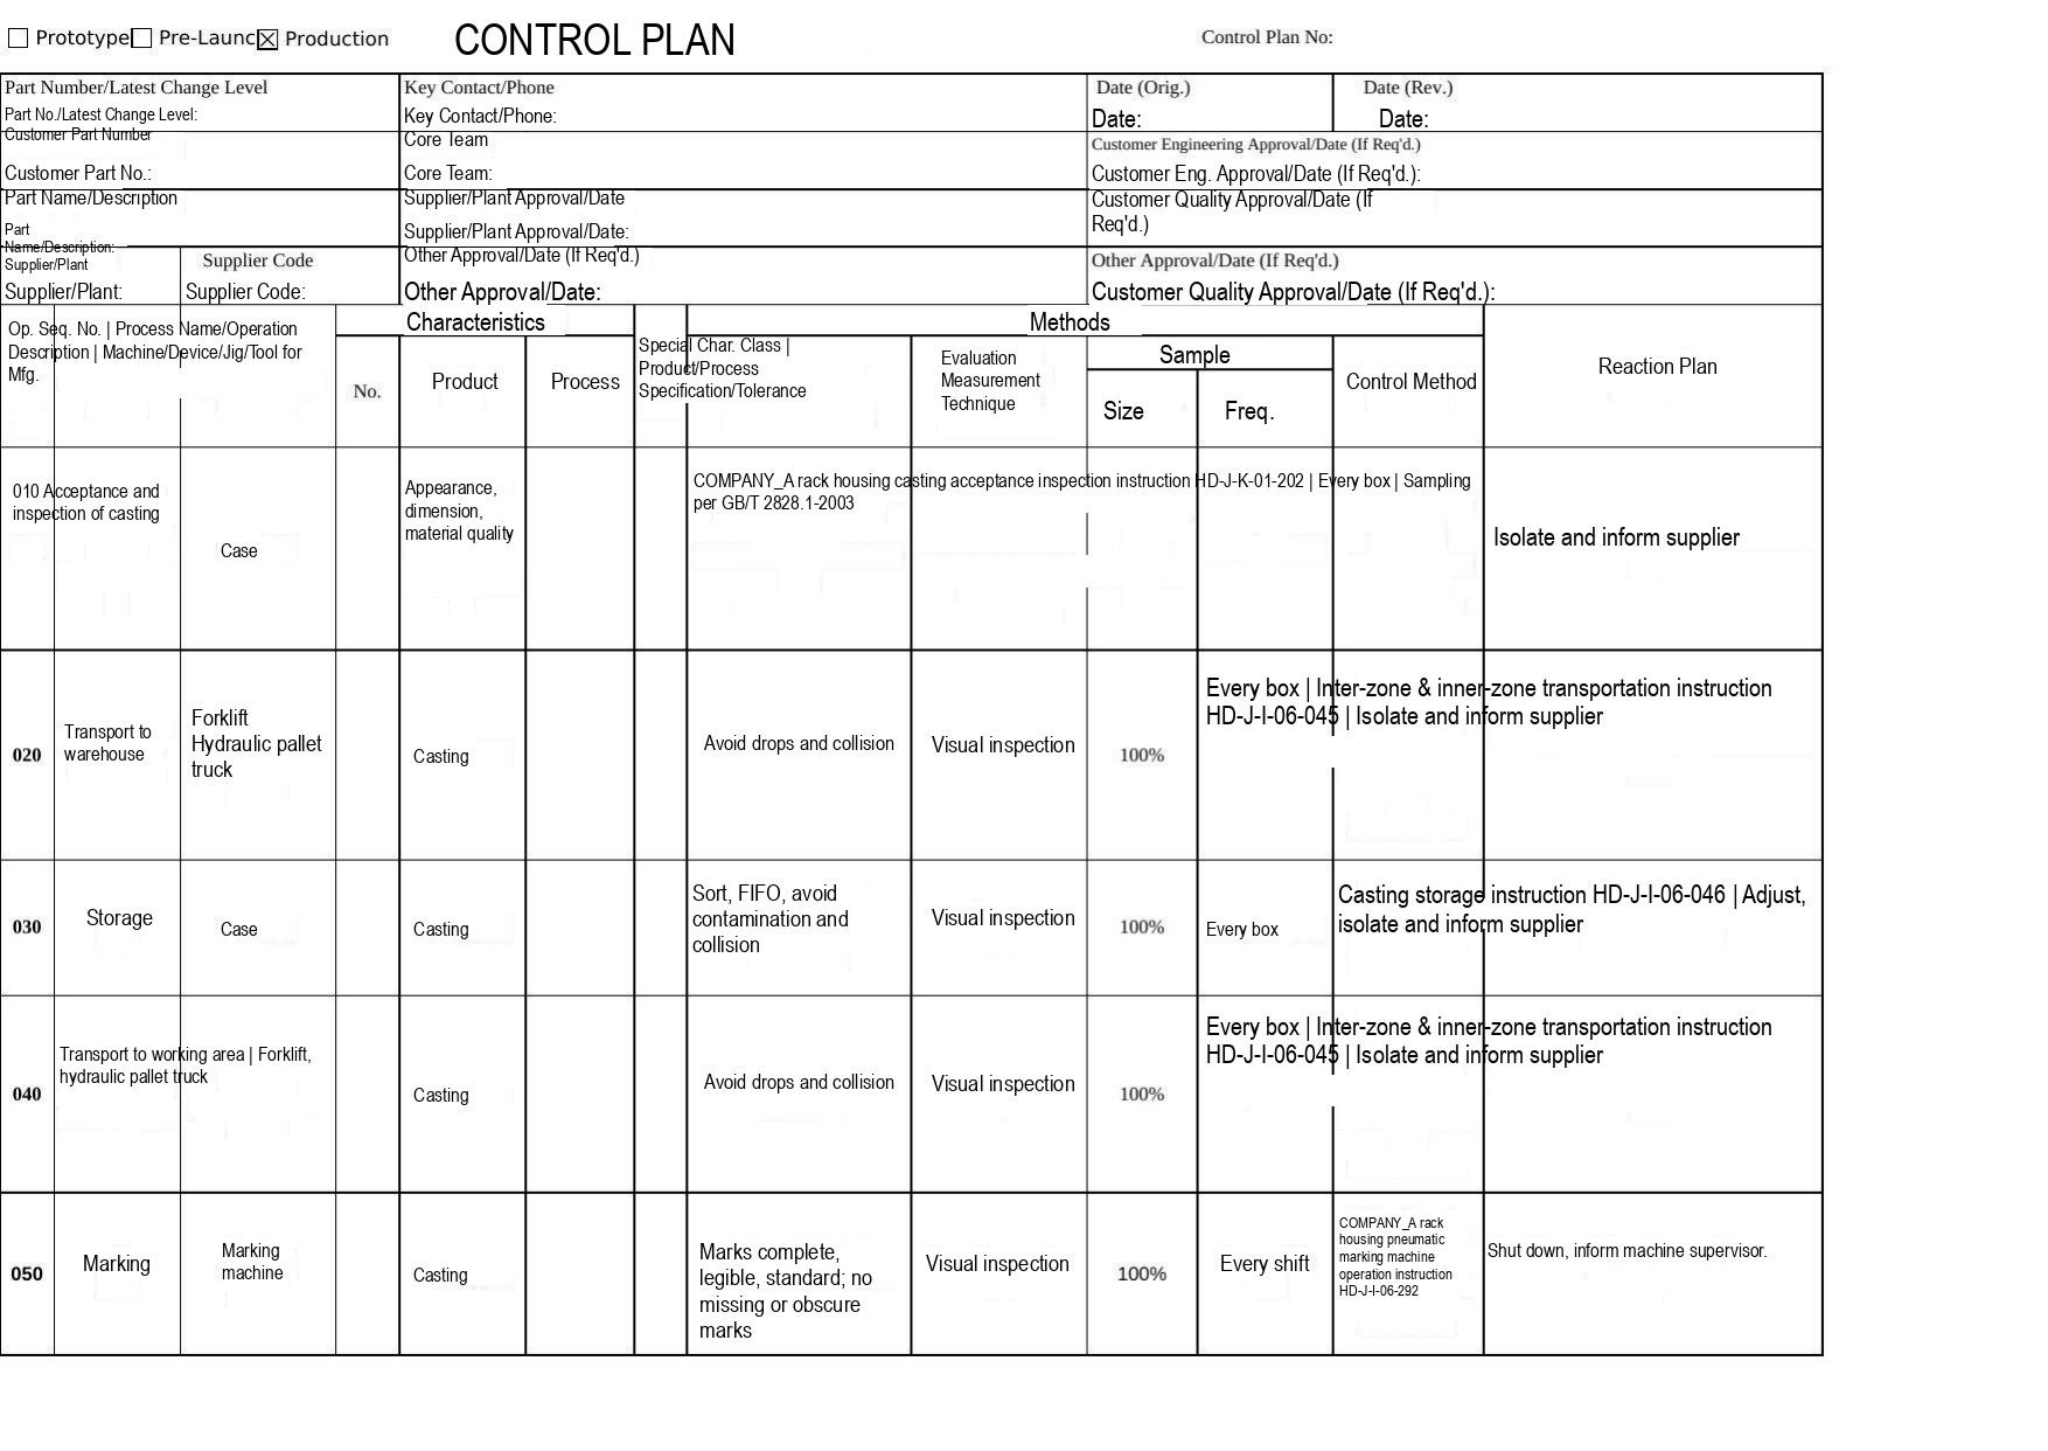☐ Prototype ☐ Pre-Launc ☒ Production

CONTROL PLAN

Control Plan No:

| Part Number/Latest Change Level<br>Part No./Latest Change Level: | Key Contact/Phone<br>Key Contact/Phone: | Date (Orig.)<br>Date: | Date (Rev.)<br>Date: |
|---|---|---|---|
| Customer Part Number<br>Customer Part No.: | Core Team<br>Core Team: | Customer Engineering Approval/Date (If Req'd.)<br>Customer Eng. Approval/Date (If Req'd.): | |
| Part Name/Description<br>Part Name/Description: | Supplier/Plant Approval/Date<br>Supplier/Plant Approval/Date: | Customer Quality Approval/Date (If Req'd.) | |
| Supplier/Plant<br>Supplier/Plant: / Supplier Code<br>Supplier Code: | Other Approval/Date (If Req'd.)<br>Other Approval/Date: | Other Approval/Date (If Req'd.)<br>Customer Quality Approval/Date (If Req'd.): | |

| Op. Seq. No. \| Process Name/Operation Description \| Machine/Device/Jig/Tool for Mfg. | | | Characteristics: No. | Characteristics: Product | Characteristics: Process | Special Char. Class \| Product/Process Specification/Tolerance | | Methods: Evaluation Measurement Technique | Methods: Sample Size | Methods: Sample Freq. | Methods: Control Method | Reaction Plan |
|---|---|---|---|---|---|---|---|---|---|---|---|---|
| 010 Acceptance and inspection of casting | | Case | | Appearance, dimension, material quality | | | COMPANY_A rack housing casting acceptance inspection instruction HD-J-K-01-202 \| Every box \| Sampling per GB/T 2828.1-2003 | | | | | Isolate and inform supplier |
| 020 | Transport to warehouse | Forklift Hydraulic pallet truck | | Casting | | | Avoid drops and collision | Visual inspection | 100% | Every box \| Inter-zone & inner-zone transportation instruction HD-J-I-06-045 \| Isolate and inform supplier | | |
| 030 | Storage | Case | | Casting | | | Sort, FIFO, avoid contamination and collision | Visual inspection | 100% | Every box | Casting storage instruction HD-J-I-06-046 \| Adjust, isolate and inform supplier | |
| 040 | Transport to working area \| Forklift, hydraulic pallet truck | | | Casting | | | Avoid drops and collision | Visual inspection | 100% | Every box \| Inter-zone & inner-zone transportation instruction HD-J-I-06-045 \| Isolate and inform supplier | | |
| 050 | Marking | Marking machine | | Casting | | | Marks complete, legible, standard; no missing or obscure marks | Visual inspection | 100% | Every shift | COMPANY_A rack housing pneumatic marking machine operation instruction HD-J-I-06-292 | Shut down, inform machine supervisor. |
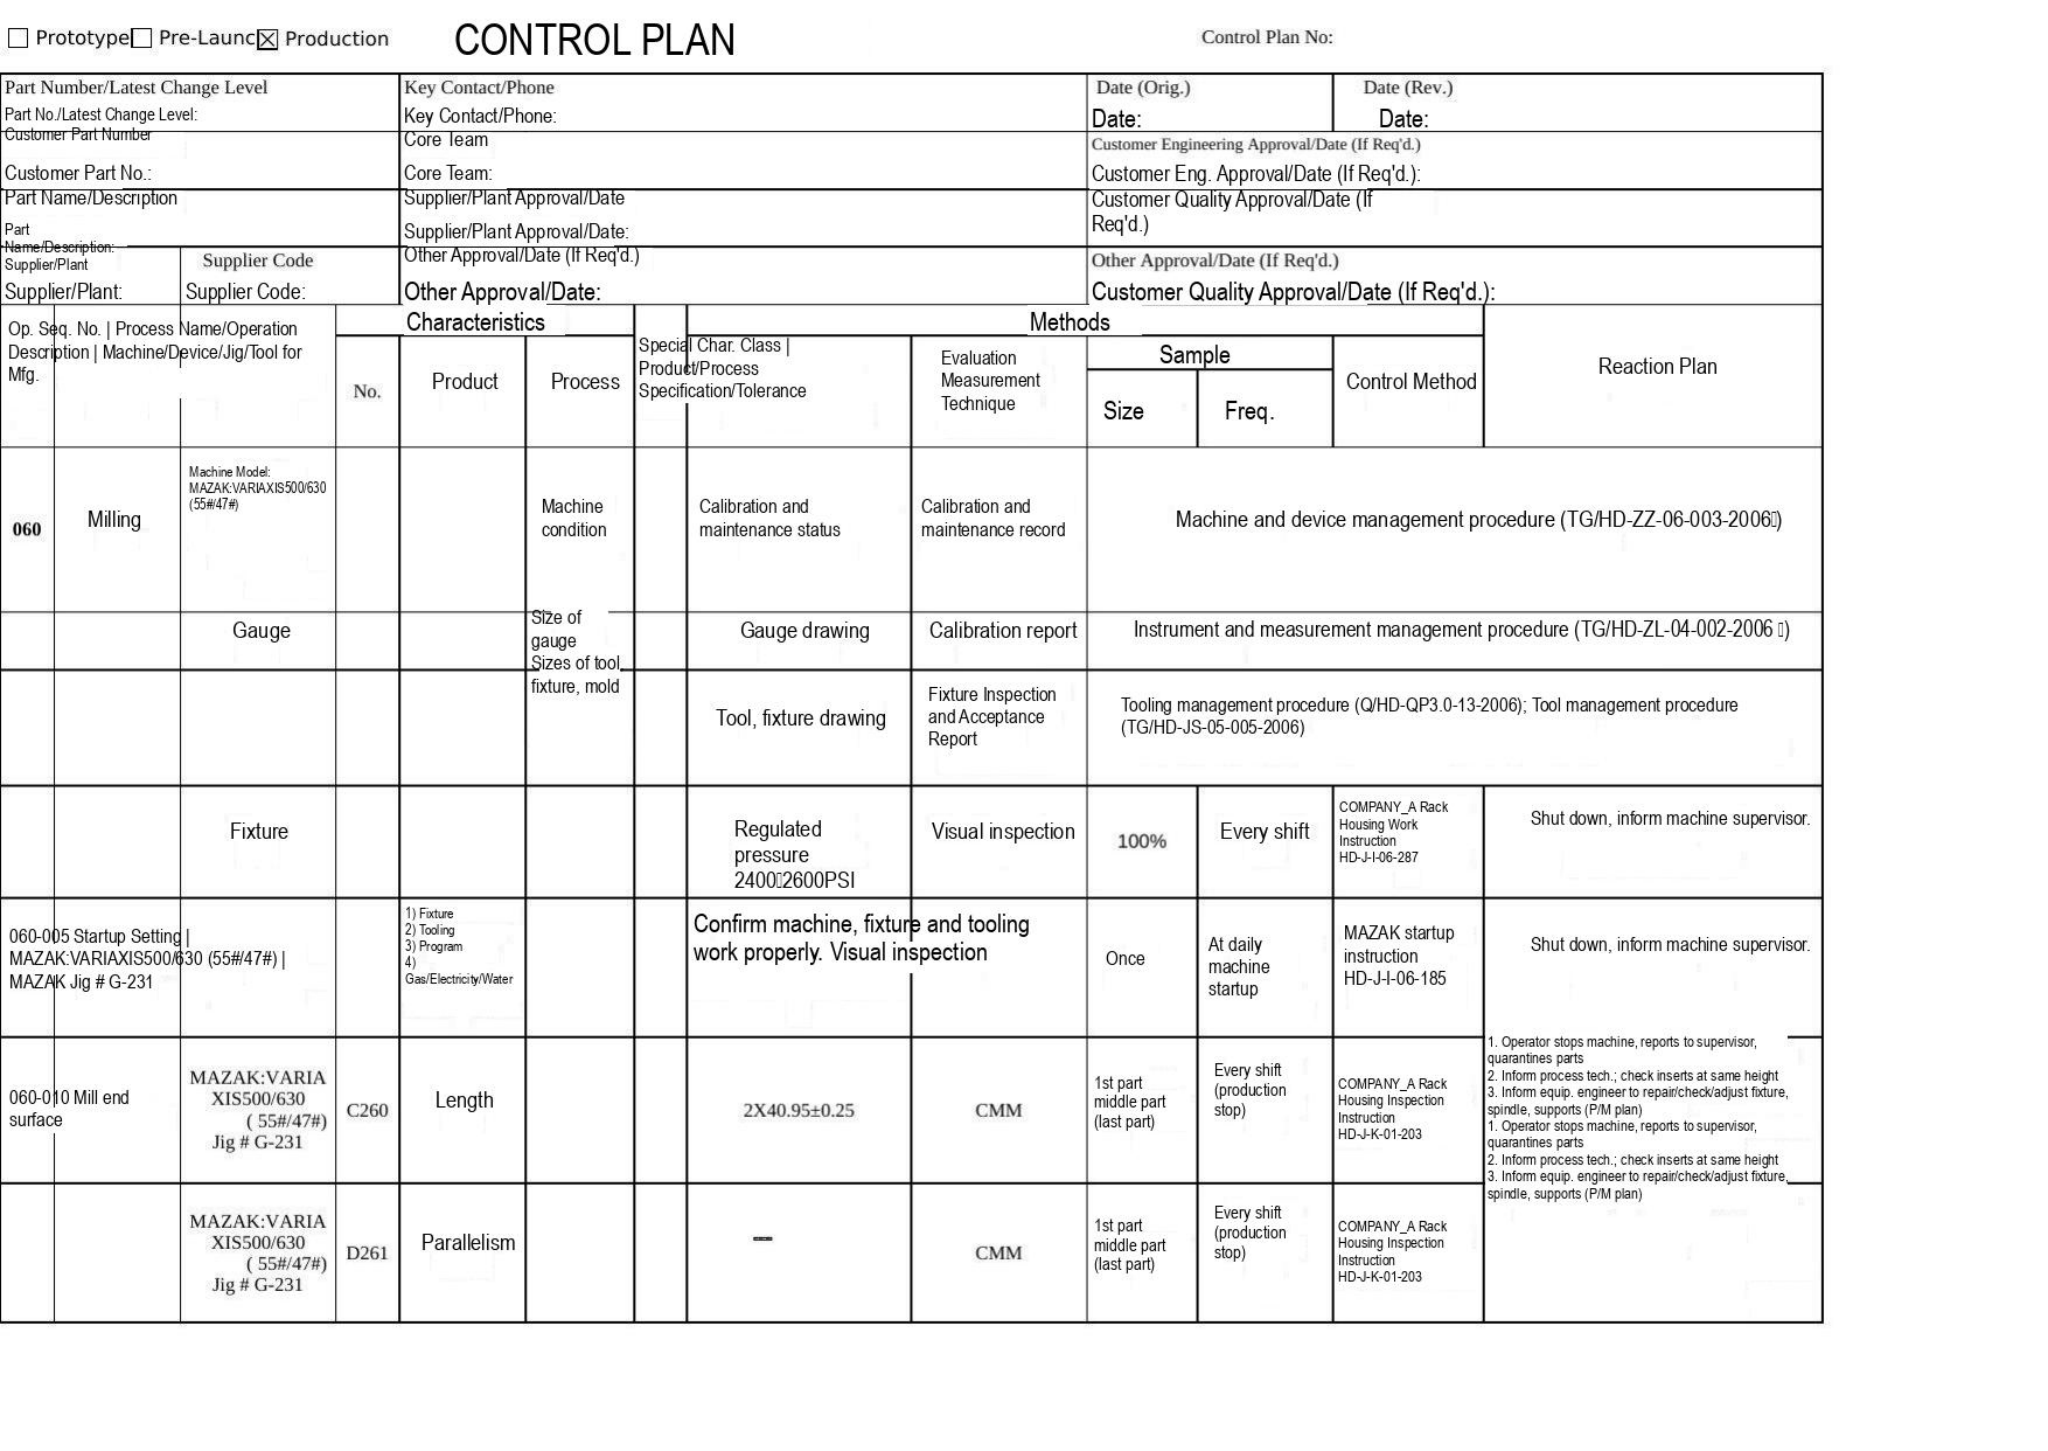☐ Prototype ☐ Pre-Launc ☒ Production

# CONTROL PLAN

Control Plan No:

| Part Number/Latest Change Level<br>Part No./Latest Change Level: | Key Contact/Phone<br>Key Contact/Phone: | Date (Orig.)<br>Date: | Date (Rev.)<br>Date: |
|---|---|---|---|
| Customer Part Number<br>Customer Part No.: | Core Team<br>Core Team: | Customer Engineering Approval/Date (If Req'd.)<br>Customer Eng. Approval/Date (If Req'd.): | |
| Part Name/Description<br>Part Name/Description: | Supplier/Plant Approval/Date<br>Supplier/Plant Approval/Date: | Customer Quality Approval/Date (If Req'd.) | |
| Supplier/Plant<br>Supplier/Plant: / Supplier Code<br>Supplier Code: | Other Approval/Date (If Req'd.)<br>Other Approval/Date: | Other Approval/Date (If Req'd.)<br>Customer Quality Approval/Date (If Req'd.): | |

| Op. Seq. No. \| Process Name/Operation Description \| Machine/Device/Jig/Tool for Mfg. | | | Characteristics No. | Characteristics Product | Characteristics Process | Special Char. Class \| Product/Process Specification/Tolerance | | Methods Evaluation Measurement Technique | Sample Size | Sample Freq. | Control Method | Reaction Plan |
|---|---|---|---|---|---|---|---|---|---|---|---|---|
| 060 | Milling | Machine Model: MAZAK:VARIAXIS500/630 (55#/47#) | | | Machine condition | | Calibration and maintenance status | Calibration and maintenance record | Machine and device management procedure (TG/HD-ZZ-06-003-2006) | | | |
| | | Gauge | | | Size of gauge | | Gauge drawing | Calibration report | Instrument and measurement management procedure (TG/HD-ZL-04-002-2006 ) | | | |
| | | | | | Sizes of tool, fixture, mold | | Tool, fixture drawing | Fixture Inspection and Acceptance Report | Tooling management procedure (Q/HD-QP3.0-13-2006); Tool management procedure (TG/HD-JS-05-005-2006) | | | |
| | | Fixture | | | | | Regulated pressure 24002600PSI | Visual inspection | 100% | Every shift | COMPANY_A Rack Housing Work Instruction HD-J-I-06-287 | Shut down, inform machine supervisor. |
| 060-005 Startup Setting \| MAZAK:VARIAXIS500/630 (55#/47#) \| MAZAK Jig # G-231 | | | | 1) Fixture<br>2) Tooling<br>3) Program<br>4) Gas/Electricity/Water | | | Confirm machine, fixture and tooling work properly. Visual inspection | | Once | At daily machine startup | MAZAK startup instruction HD-J-I-06-185 | Shut down, inform machine supervisor. |
| 060-010 Mill end surface | | MAZAK:VARIAXIS500/630 ( 55#/47#) Jig # G-231 | C260 | Length | | | 2X40.95±0.25 | CMM | 1st part middle part (last part) | Every shift (production stop) | COMPANY_A Rack Housing Inspection Instruction HD-J-K-01-203 | 1. Operator stops machine, reports to supervisor, quarantines parts<br>2. Inform process tech.; check inserts at same height<br>3. Inform equip. engineer to repair/check/adjust fixture, spindle, supports (P/M plan) |
| | | MAZAK:VARIAXIS500/630 ( 55#/47#) Jig # G-231 | D261 | Parallelism | | | — | CMM | 1st part middle part (last part) | Every shift (production stop) | COMPANY_A Rack Housing Inspection Instruction HD-J-K-01-203 | 1. Operator stops machine, reports to supervisor, quarantines parts<br>2. Inform process tech.; check inserts at same height<br>3. Inform equip. engineer to repair/check/adjust fixture, spindle, supports (P/M plan) |
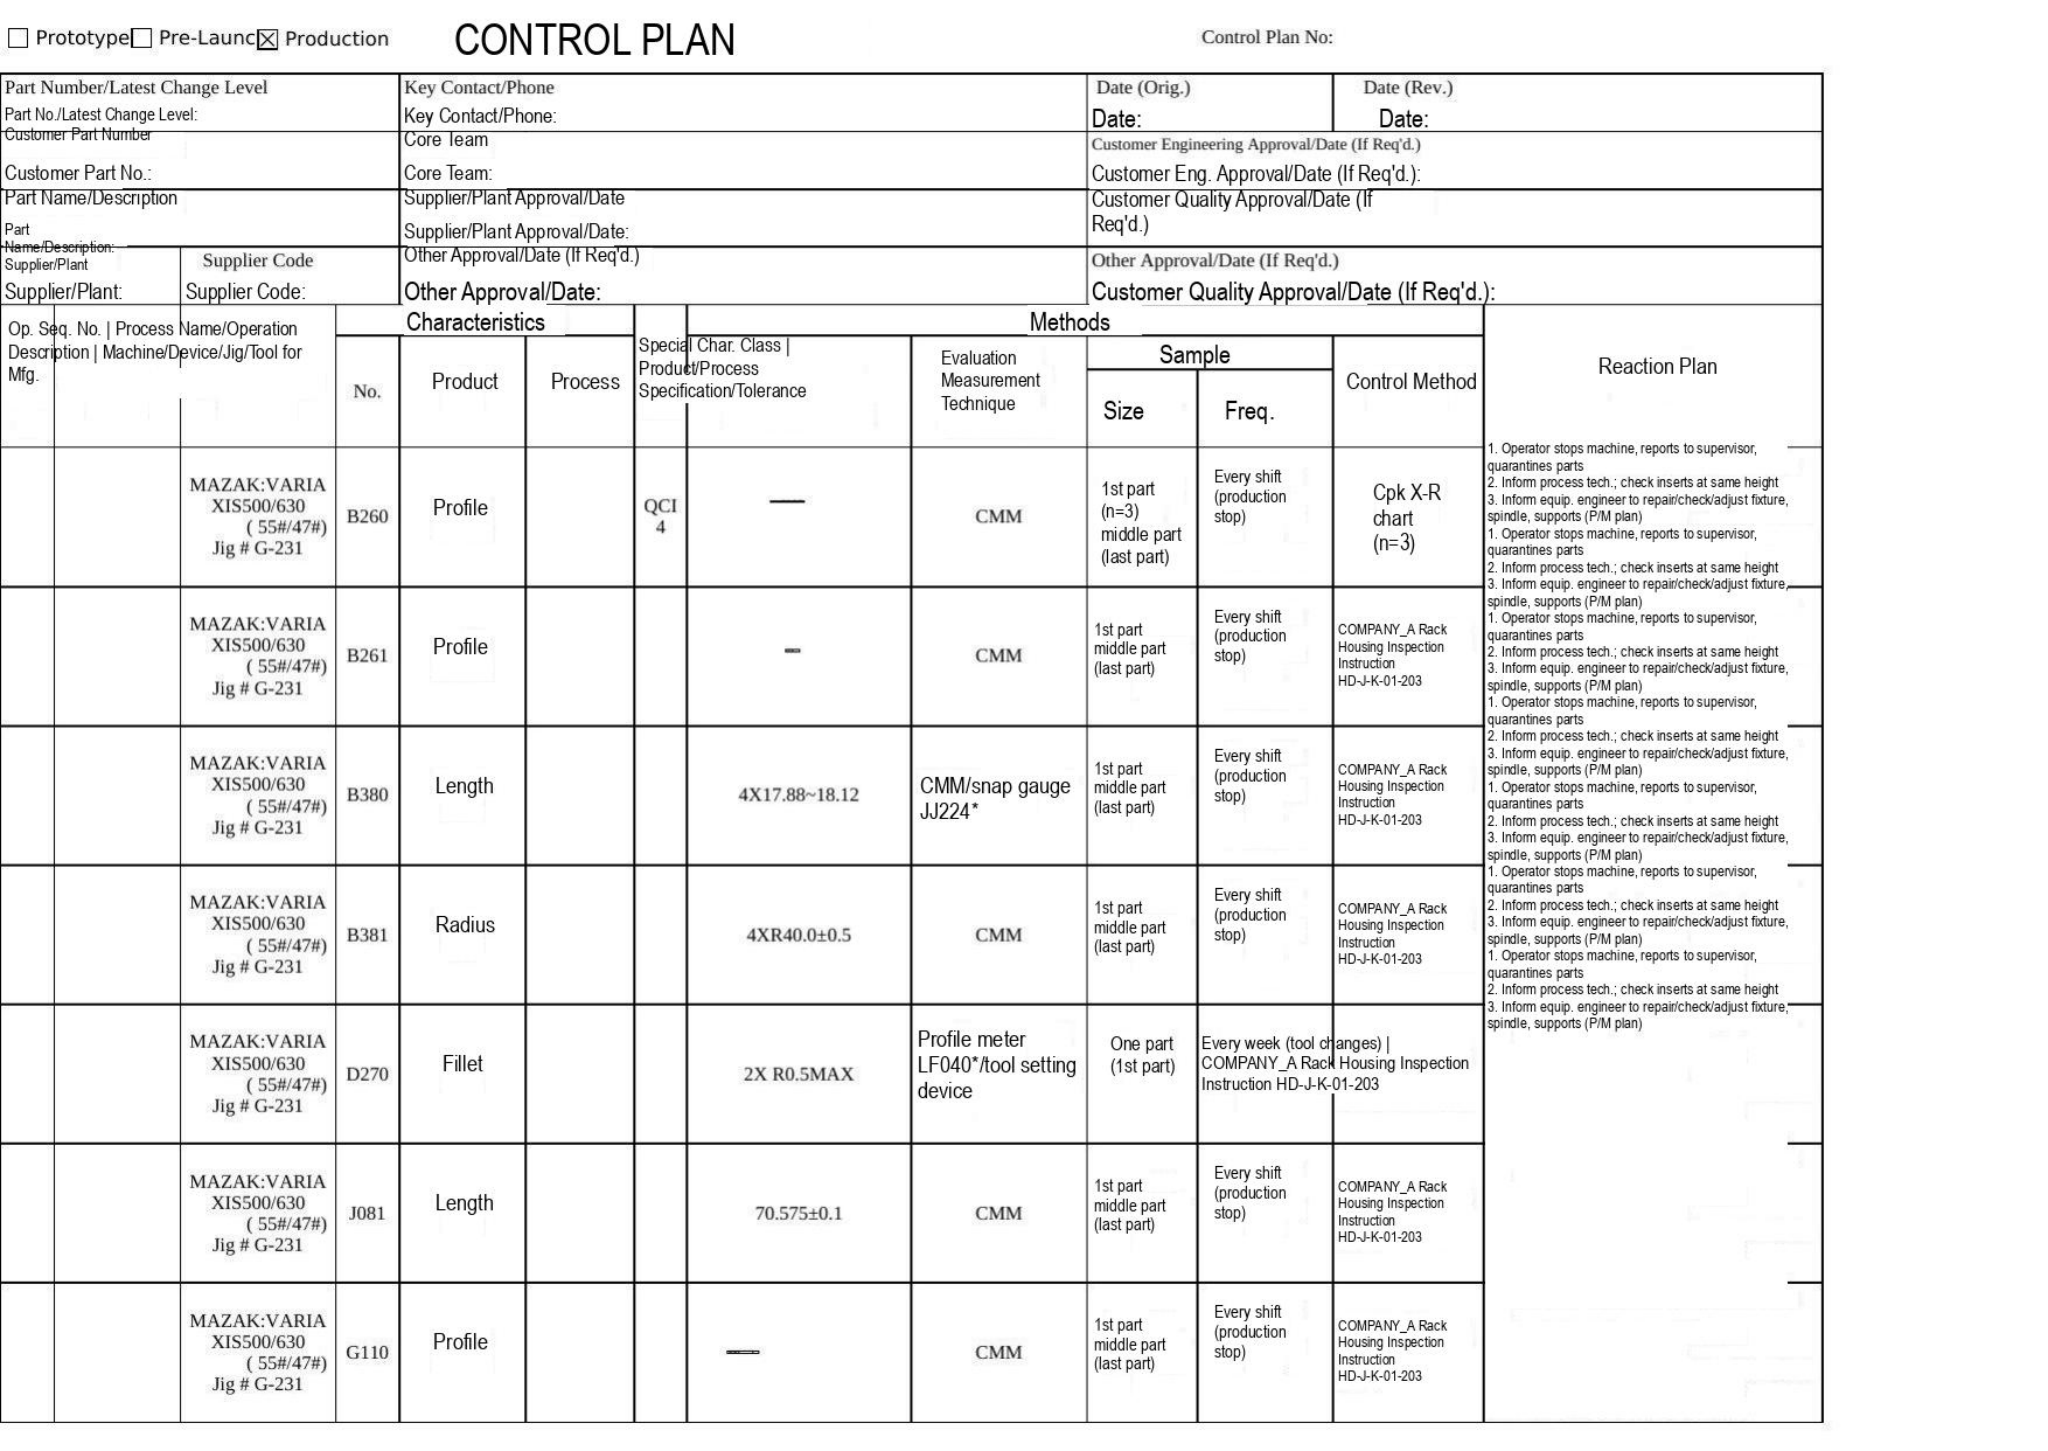☐ Prototype☐ Pre-Launc☒ Production

# CONTROL PLAN

Control Plan No:

| Part Number/Latest Change Level<br>Part No./Latest Change Level: | | Key Contact/Phone<br>Key Contact/Phone: | Date (Orig.)<br>Date: | Date (Rev.)<br>Date: |
|---|---|---|---|---|
| Customer Part Number<br>Customer Part No.: | | Core Team<br>Core Team: | Customer Engineering Approval/Date (If Req'd.)<br>Customer Eng. Approval/Date (If Req'd.): | |
| Part Name/Description<br>Part Name/Description: | | Supplier/Plant Approval/Date<br>Supplier/Plant Approval/Date: | Customer Quality Approval/Date (If Req'd.) | |
| Supplier/Plant<br>Supplier/Plant: | Supplier Code<br>Supplier Code: | Other Approval/Date (If Req'd.)<br>Other Approval/Date: | Other Approval/Date (If Req'd.)<br>Customer Quality Approval/Date (If Req'd.): | |

| Op. Seq. No. \| Process Name/Operation Description \| Machine/Device/Jig/Tool for Mfg. | | | Characteristics: No. | Characteristics: Product | Characteristics: Process | Special Char. Class \| Product/Process Specification/Tolerance | | Methods: Evaluation Measurement Technique | Sample: Size | Sample: Freq. | Control Method | Reaction Plan |
|---|---|---|---|---|---|---|---|---|---|---|---|---|
| | | MAZAK:VARIA XIS500/630 ( 55#/47#) Jig # G-231 | B260 | Profile | | QCI 4 | — | CMM | 1st part (n=3) middle part (last part) | Every shift (production stop) | Cpk X-R chart (n=3) | 1. Operator stops machine, reports to supervisor, quarantines parts<br>2. Inform process tech.; check inserts at same height<br>3. Inform equip. engineer to repair/check/adjust fixture, spindle, supports (P/M plan) |
| | | MAZAK:VARIA XIS500/630 ( 55#/47#) Jig # G-231 | B261 | Profile | | | — | CMM | 1st part middle part (last part) | Every shift (production stop) | COMPANY_A Rack Housing Inspection Instruction HD-J-K-01-203 | 1. Operator stops machine, reports to supervisor, quarantines parts<br>2. Inform process tech.; check inserts at same height<br>3. Inform equip. engineer to repair/check/adjust fixture, spindle, supports (P/M plan) |
| | | MAZAK:VARIA XIS500/630 ( 55#/47#) Jig # G-231 | B380 | Length | | | 4X17.88~18.12 | CMM/snap gauge JJ224* | 1st part middle part (last part) | Every shift (production stop) | COMPANY_A Rack Housing Inspection Instruction HD-J-K-01-203 | 1. Operator stops machine, reports to supervisor, quarantines parts<br>2. Inform process tech.; check inserts at same height<br>3. Inform equip. engineer to repair/check/adjust fixture, spindle, supports (P/M plan) |
| | | MAZAK:VARIA XIS500/630 ( 55#/47#) Jig # G-231 | B381 | Radius | | | 4XR40.0±0.5 | CMM | 1st part middle part (last part) | Every shift (production stop) | COMPANY_A Rack Housing Inspection Instruction HD-J-K-01-203 | 1. Operator stops machine, reports to supervisor, quarantines parts<br>2. Inform process tech.; check inserts at same height<br>3. Inform equip. engineer to repair/check/adjust fixture, spindle, supports (P/M plan) |
| | | MAZAK:VARIA XIS500/630 ( 55#/47#) Jig # G-231 | D270 | Fillet | | | 2X R0.5MAX | Profile meter LF040*/tool setting device | One part (1st part) | Every week (tool changes) \| COMPANY_A Rack Housing Inspection Instruction HD-J-K-01-203 | | 1. Operator stops machine, reports to supervisor, quarantines parts<br>2. Inform process tech.; check inserts at same height<br>3. Inform equip. engineer to repair/check/adjust fixture, spindle, supports (P/M plan) |
| | | MAZAK:VARIA XIS500/630 ( 55#/47#) Jig # G-231 | J081 | Length | | | 70.575±0.1 | CMM | 1st part middle part (last part) | Every shift (production stop) | COMPANY_A Rack Housing Inspection Instruction HD-J-K-01-203 | 1. Operator stops machine, reports to supervisor, quarantines parts<br>2. Inform process tech.; check inserts at same height<br>3. Inform equip. engineer to repair/check/adjust fixture, spindle, supports (P/M plan) |
| | | MAZAK:VARIA XIS500/630 ( 55#/47#) Jig # G-231 | G110 | Profile | | | — | CMM | 1st part middle part (last part) | Every shift (production stop) | COMPANY_A Rack Housing Inspection Instruction HD-J-K-01-203 | 1. Operator stops machine, reports to supervisor, quarantines parts<br>2. Inform process tech.; check inserts at same height<br>3. Inform equip. engineer to repair/check/adjust fixture, spindle, supports (P/M plan) |
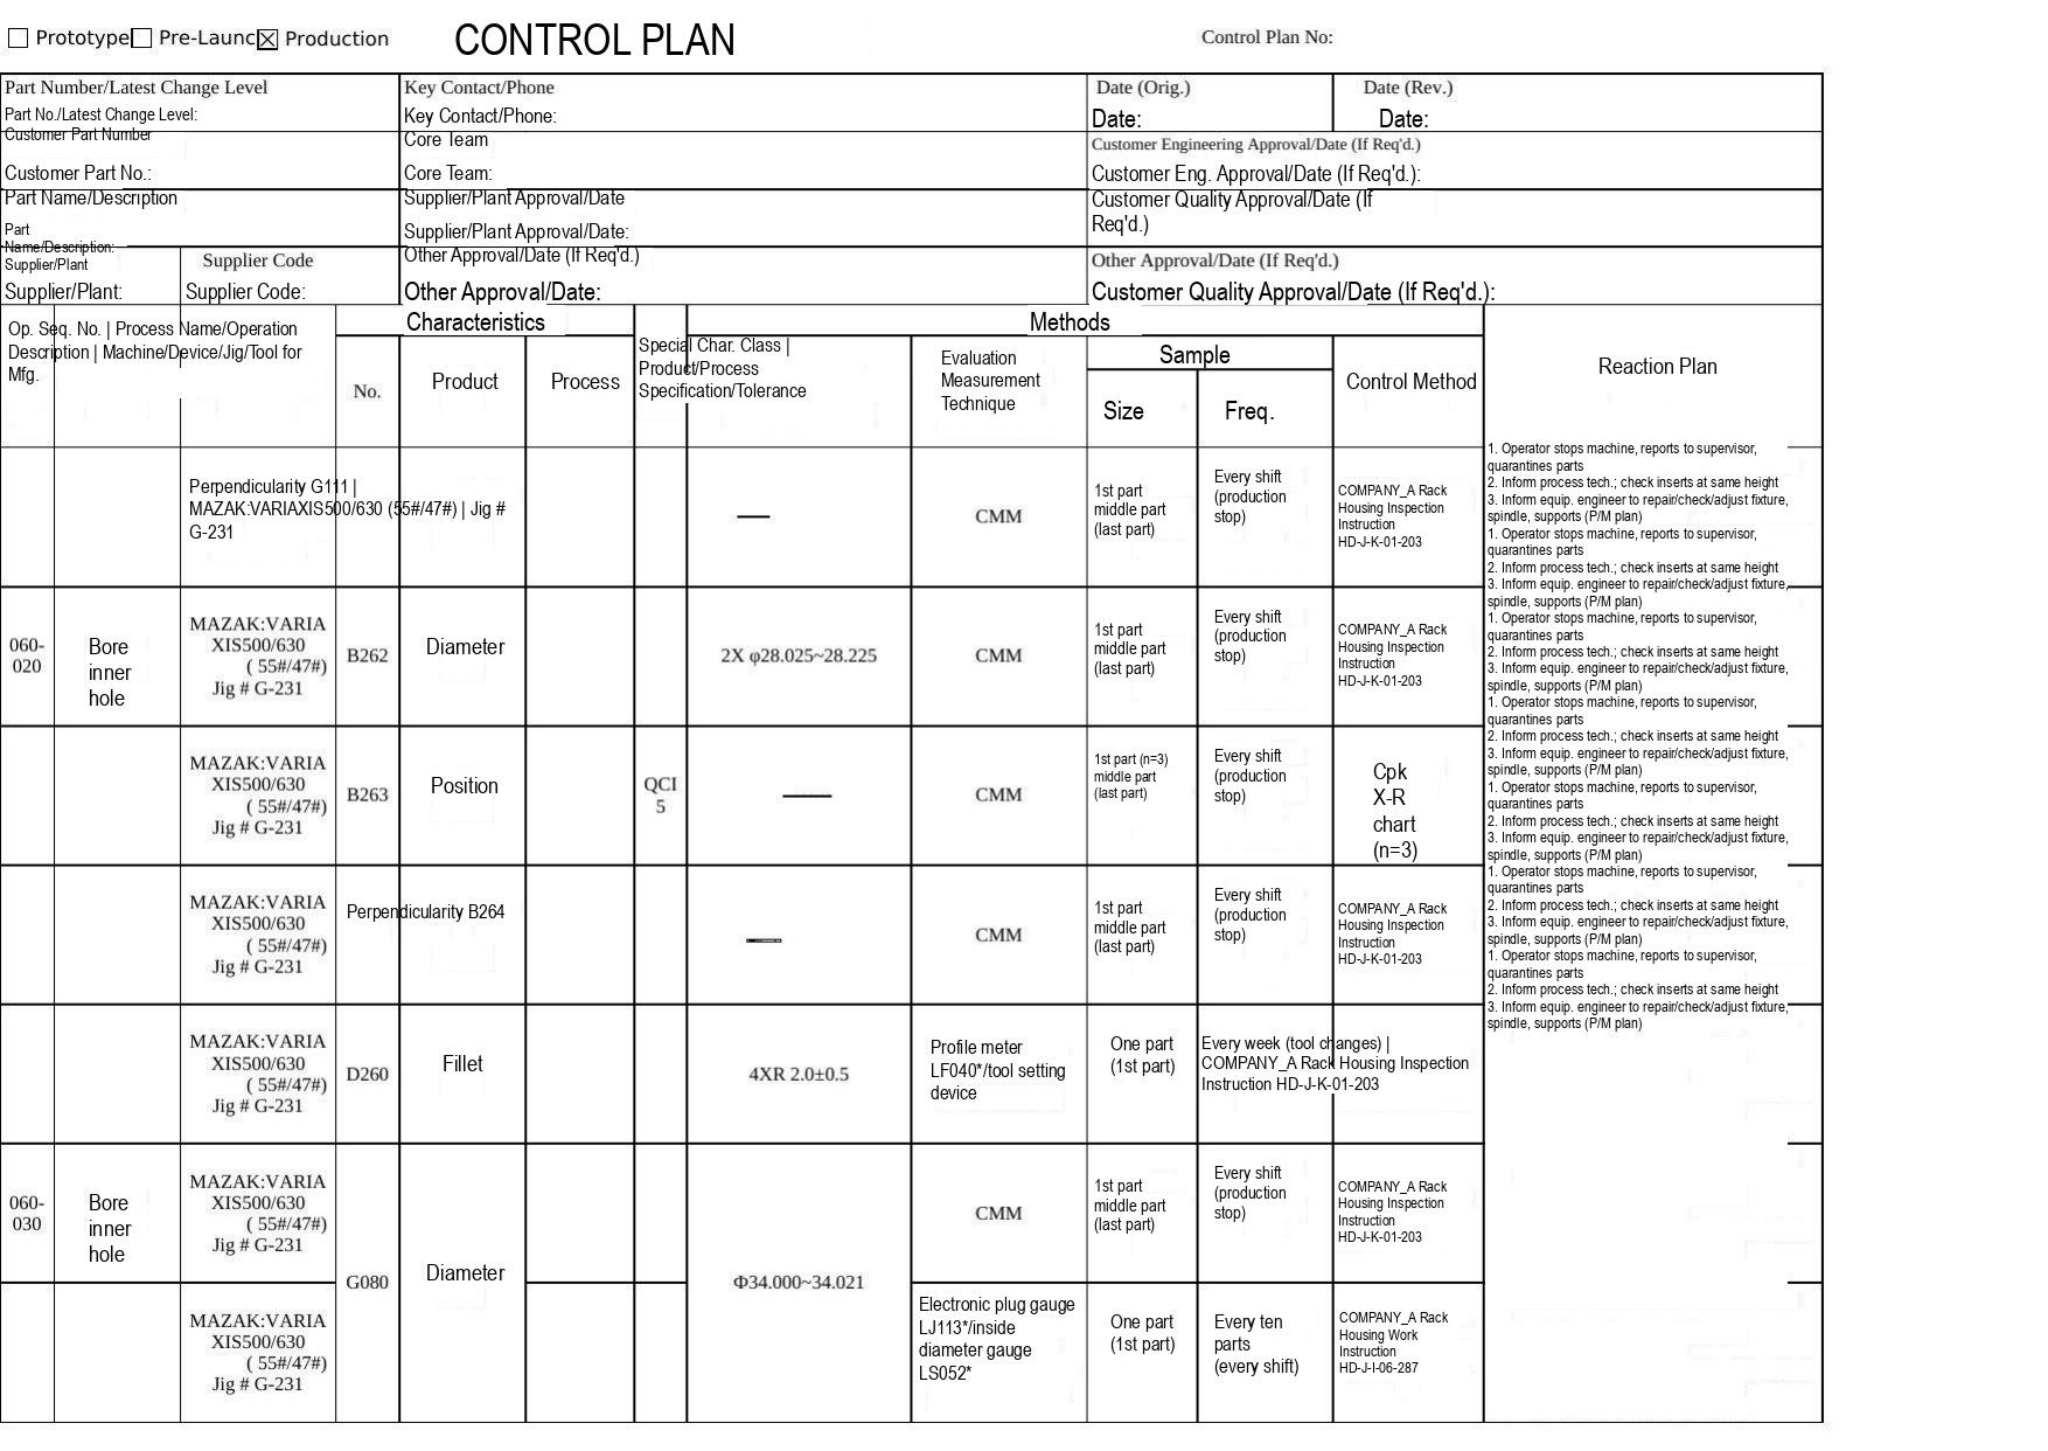☐ Prototype☐ Pre-Launc☒ Production

CONTROL PLAN

Control Plan No:

| Part Number/Latest Change Level<br>Part No./Latest Change Level: | | Key Contact/Phone<br>Key Contact/Phone: | Date (Orig.)<br>Date: | Date (Rev.)<br>Date: |
|---|---|---|---|---|
| Customer Part Number<br>Customer Part No.: | | Core Team<br>Core Team: | Customer Engineering Approval/Date (If Req'd.)<br>Customer Eng. Approval/Date (If Req'd.): | |
| Part Name/Description<br>Part Name/Description: | | Supplier/Plant Approval/Date<br>Supplier/Plant Approval/Date: | Customer Quality Approval/Date (If Req'd.) | |
| Supplier/Plant<br>Supplier/Plant: | Supplier Code<br>Supplier Code: | Other Approval/Date (If Req'd.)<br>Other Approval/Date: | Other Approval/Date (If Req'd.)<br>Customer Quality Approval/Date (If Req'd.): | |

| Op. Seq. No. | Process Name/Operation Description | Machine/Device/Jig/Tool for Mfg. | Characteristics No. | Characteristics Product | Characteristics Process | Special Char. Class | Methods Product/Process Specification/Tolerance | Methods Evaluation Measurement Technique | Methods Sample Size | Methods Sample Freq. | Methods Control Method | Reaction Plan |
|---|---|---|---|---|---|---|---|---|---|---|---|---|
| | | Perpendicularity G111 \| MAZAK:VARIAXIS500/630 (55#/47#) \| Jig # G-231 | | | | | — | CMM | 1st part middle part (last part) | Every shift (production stop) | COMPANY_A Rack Housing Inspection Instruction HD-J-K-01-203 | 1. Operator stops machine, reports to supervisor, quarantines parts<br>2. Inform process tech.; check inserts at same height<br>3. Inform equip. engineer to repair/check/adjust fixture, spindle, supports (P/M plan)<br>1. Operator stops machine, reports to supervisor, quarantines parts<br>2. Inform process tech.; check inserts at same height<br>3. Inform equip. engineer to repair/check/adjust fixture, spindle, supports (P/M plan) |
| 060-020 | Bore inner hole | MAZAK:VARIAXIS500/630 ( 55#/47#) Jig # G-231 | B262 | Diameter | | | 2X φ28.025~28.225 | CMM | 1st part middle part (last part) | Every shift (production stop) | COMPANY_A Rack Housing Inspection Instruction HD-J-K-01-203 | 1. Operator stops machine, reports to supervisor, quarantines parts<br>2. Inform process tech.; check inserts at same height<br>3. Inform equip. engineer to repair/check/adjust fixture, spindle, supports (P/M plan)<br>1. Operator stops machine, reports to supervisor, quarantines parts<br>2. Inform process tech.; check inserts at same height<br>3. Inform equip. engineer to repair/check/adjust fixture, spindle, supports (P/M plan) |
| | | MAZAK:VARIAXIS500/630 ( 55#/47#) Jig # G-231 | B263 | Position | | QCI 5 | — | CMM | 1st part (n=3) middle part (last part) | Every shift (production stop) | Cpk X-R chart (n=3) | 1. Operator stops machine, reports to supervisor, quarantines parts<br>2. Inform process tech.; check inserts at same height<br>3. Inform equip. engineer to repair/check/adjust fixture, spindle, supports (P/M plan) |
| | | MAZAK:VARIAXIS500/630 ( 55#/47#) Jig # G-231 | Perpendicularity B264 | | | | — | CMM | 1st part middle part (last part) | Every shift (production stop) | COMPANY_A Rack Housing Inspection Instruction HD-J-K-01-203 | 1. Operator stops machine, reports to supervisor, quarantines parts<br>2. Inform process tech.; check inserts at same height<br>3. Inform equip. engineer to repair/check/adjust fixture, spindle, supports (P/M plan)<br>1. Operator stops machine, reports to supervisor, quarantines parts<br>2. Inform process tech.; check inserts at same height<br>3. Inform equip. engineer to repair/check/adjust fixture, spindle, supports (P/M plan) |
| | | MAZAK:VARIAXIS500/630 ( 55#/47#) Jig # G-231 | D260 | Fillet | | | 4XR 2.0±0.5 | Profile meter LF040*/tool setting device | One part (1st part) | Every week (tool changes) \| COMPANY_A Rack Housing Inspection Instruction HD-J-K-01-203 | | |
| 060-030 | Bore inner hole | MAZAK:VARIAXIS500/630 ( 55#/47#) Jig # G-231 | G080 | Diameter | | | Φ34.000~34.021 | CMM | 1st part middle part (last part) | Every shift (production stop) | COMPANY_A Rack Housing Inspection Instruction HD-J-K-01-203 | |
| | | MAZAK:VARIAXIS500/630 ( 55#/47#) Jig # G-231 | | | | | | Electronic plug gauge LJ113*/inside diameter gauge LS052* | One part (1st part) | Every ten parts (every shift) | COMPANY_A Rack Housing Work Instruction HD-J-I-06-287 | |
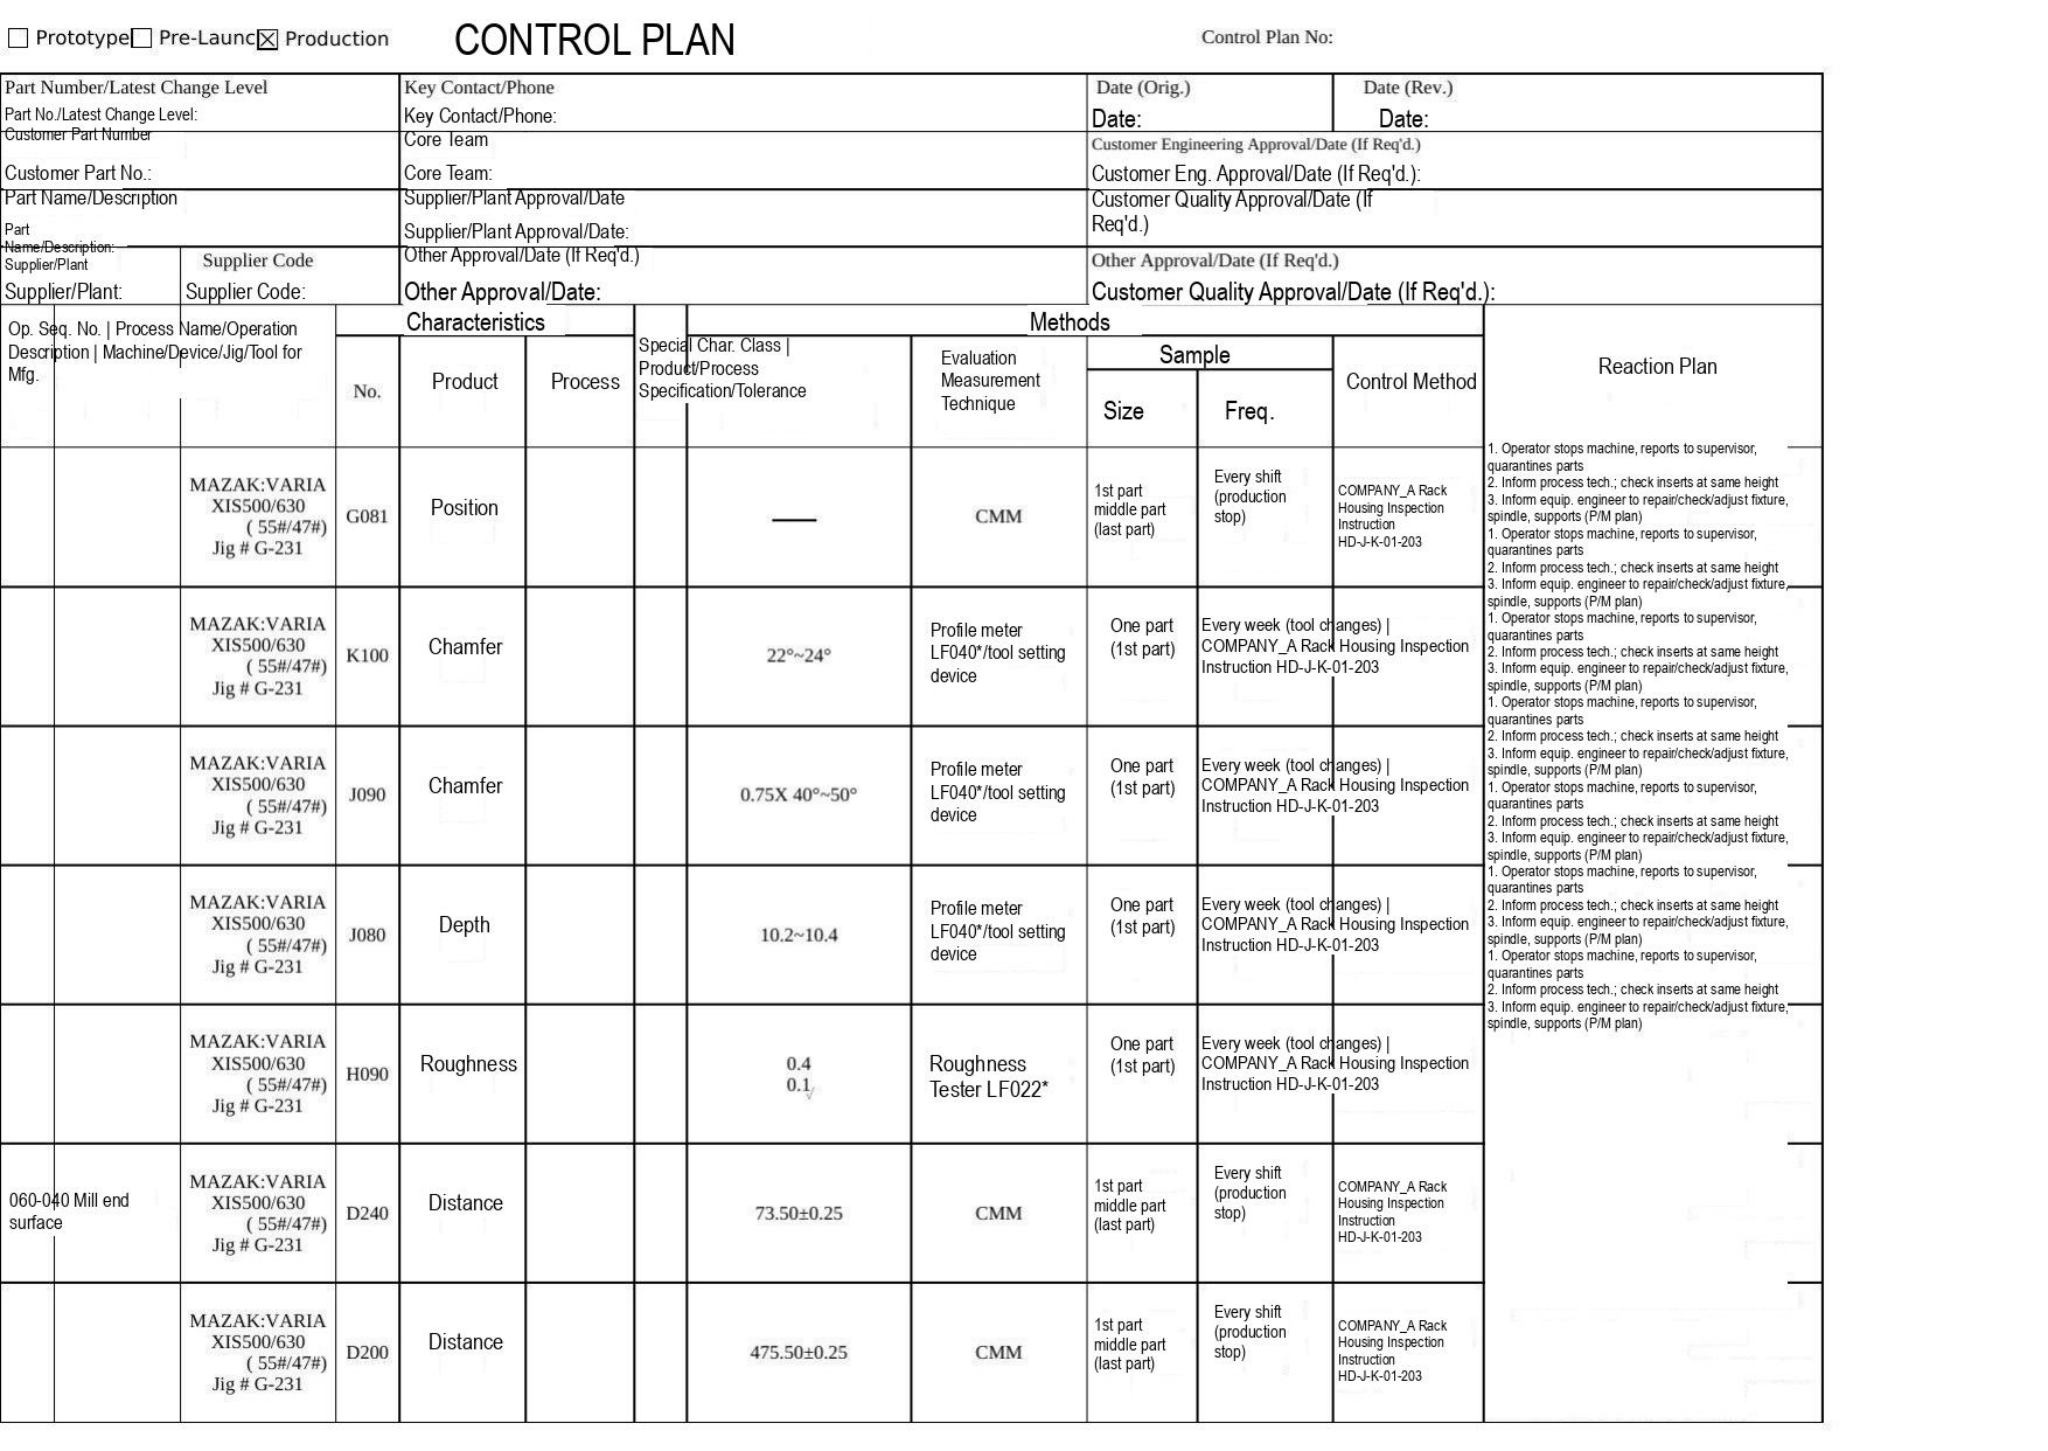☐ Prototype☐ Pre-Launc☒ Production

# CONTROL PLAN

Control Plan No:

| Part Number/Latest Change Level<br>Part No./Latest Change Level: | Key Contact/Phone<br>Key Contact/Phone: | Date (Orig.)<br>Date: | Date (Rev.)<br>Date: |
|---|---|---|---|
| Customer Part Number<br>Customer Part No.: | Core Team<br>Core Team: | Customer Engineering Approval/Date (If Req'd.)<br>Customer Eng. Approval/Date (If Req'd.): | |
| Part Name/Description<br>Part Name/Description: | Supplier/Plant Approval/Date<br>Supplier/Plant Approval/Date: | Customer Quality Approval/Date (If Req'd.) | |
| Supplier/Plant<br>Supplier/Plant: — Supplier Code<br>Supplier Code: | Other Approval/Date (If Req'd.)<br>Other Approval/Date: | Other Approval/Date (If Req'd.)<br>Customer Quality Approval/Date (If Req'd.): | |

| Op. Seq. No. | Process Name/Operation Description | Machine/Device/Jig/Tool for Mfg. | Characteristics<br>No. | Characteristics<br>Product | Characteristics<br>Process | Special Char. Class | Product/Process Specification/Tolerance | Methods<br>Evaluation Measurement Technique | Methods<br>Sample<br>Size | Methods<br>Sample<br>Freq. | Methods<br>Control Method | Reaction Plan |
|---|---|---|---|---|---|---|---|---|---|---|---|---|
| | | MAZAK:VARIA XIS500/630 ( 55#/47#) Jig # G-231 | G081 | Position | | | — | CMM | 1st part middle part (last part) | Every shift (production stop) | COMPANY_A Rack Housing Inspection Instruction HD-J-K-01-203 | 1. Operator stops machine, reports to supervisor, quarantines parts 2. Inform process tech.; check inserts at same height 3. Inform equip. engineer to repair/check/adjust fixture, spindle, supports (P/M plan) |
| | | MAZAK:VARIA XIS500/630 ( 55#/47#) Jig # G-231 | K100 | Chamfer | | | 22°~24° | Profile meter LF040*/tool setting device | One part (1st part) | Every week (tool changes) | COMPANY_A Rack Housing Inspection Instruction HD-J-K-01-203 | 1. Operator stops machine, reports to supervisor, quarantines parts 2. Inform process tech.; check inserts at same height 3. Inform equip. engineer to repair/check/adjust fixture, spindle, supports (P/M plan) |
| | | MAZAK:VARIA XIS500/630 ( 55#/47#) Jig # G-231 | J090 | Chamfer | | | 0.75X 40°~50° | Profile meter LF040*/tool setting device | One part (1st part) | Every week (tool changes) | COMPANY_A Rack Housing Inspection Instruction HD-J-K-01-203 | 1. Operator stops machine, reports to supervisor, quarantines parts 2. Inform process tech.; check inserts at same height 3. Inform equip. engineer to repair/check/adjust fixture, spindle, supports (P/M plan) |
| | | MAZAK:VARIA XIS500/630 ( 55#/47#) Jig # G-231 | J080 | Depth | | | 10.2~10.4 | Profile meter LF040*/tool setting device | One part (1st part) | Every week (tool changes) | COMPANY_A Rack Housing Inspection Instruction HD-J-K-01-203 | 1. Operator stops machine, reports to supervisor, quarantines parts 2. Inform process tech.; check inserts at same height 3. Inform equip. engineer to repair/check/adjust fixture, spindle, supports (P/M plan) |
| | | MAZAK:VARIA XIS500/630 ( 55#/47#) Jig # G-231 | H090 | Roughness | | | 0.4<br>0.1 | Roughness Tester LF022* | One part (1st part) | Every week (tool changes) | COMPANY_A Rack Housing Inspection Instruction HD-J-K-01-203 | 1. Operator stops machine, reports to supervisor, quarantines parts 2. Inform process tech.; check inserts at same height 3. Inform equip. engineer to repair/check/adjust fixture, spindle, supports (P/M plan) |
| 060-040 | Mill end surface | MAZAK:VARIA XIS500/630 ( 55#/47#) Jig # G-231 | D240 | Distance | | | 73.50±0.25 | CMM | 1st part middle part (last part) | Every shift (production stop) | COMPANY_A Rack Housing Inspection Instruction HD-J-K-01-203 | 1. Operator stops machine, reports to supervisor, quarantines parts 2. Inform process tech.; check inserts at same height 3. Inform equip. engineer to repair/check/adjust fixture, spindle, supports (P/M plan) |
| | | MAZAK:VARIA XIS500/630 ( 55#/47#) Jig # G-231 | D200 | Distance | | | 475.50±0.25 | CMM | 1st part middle part (last part) | Every shift (production stop) | COMPANY_A Rack Housing Inspection Instruction HD-J-K-01-203 | 1. Operator stops machine, reports to supervisor, quarantines parts 2. Inform process tech.; check inserts at same height 3. Inform equip. engineer to repair/check/adjust fixture, spindle, supports (P/M plan) |